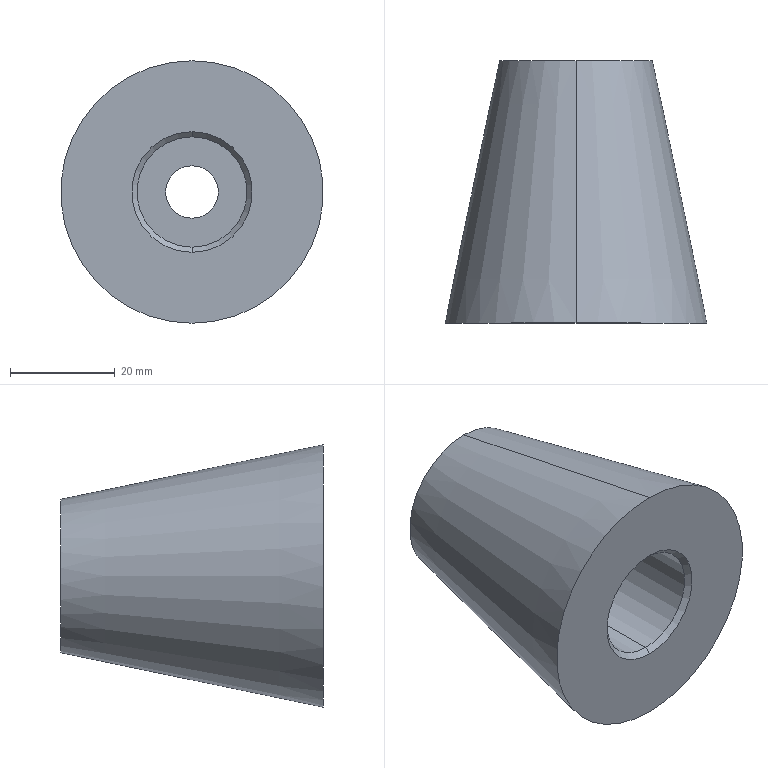Part | STEP file | ND25021-01-JDKM-05-SL | 1 solid | 13 faces | box 50 x 50 x 50 mm | volume 54211 mm3 | cone 6 | cylinder 4 | plane 3 | commonest cylinder face diameters 10 x2 21 x2
STEP:
#1=CARTESIAN_POINT('',(0.,0.,0.));
#2=DIRECTION('',(0.,0.,1.));
#3=DIRECTION('',(1.,0.,0.));
#4=AXIS2_PLACEMENT_3D('',#1,#2,#3);
#5=CARTESIAN_POINT('',(0.,1.,-10.5));
#6=VERTEX_POINT('',#5);
#7=CARTESIAN_POINT('',(0.,0.,-11.5));
#8=VERTEX_POINT('',#7);
#9=CARTESIAN_POINT('',(0.,1.,-10.5));
#10=DIRECTION('',(0.,-0.7071,-0.7071));
#11=VECTOR('',#10,1.);
#12=LINE('',#9,#11);
#13=CARTESIAN_POINT('',(0.,1.,0.));
#14=DIRECTION('',(0.,-1.,0.));
#15=DIRECTION('',(0.,0.,-1.));
#16=AXIS2_PLACEMENT_3D('',#13,#14,#15);
#17=CONICAL_SURFACE('',#16,10.5,0.7854);
#18=CARTESIAN_POINT('',(6.283,0.));
#19=DIRECTION('',(0.,1.));
#20=VECTOR('',#19,1.);
#21=LINE('',#18,#20);
#22=(GEOMETRIC_REPRESENTATION_CONTEXT(2)PARAMETRIC_REPRESENTATION_CONTEXT()REPRESENTATION_CONTEXT('',''));
#23=DEFINITIONAL_REPRESENTATION('',(#21),#22);
#24=PCURVE('',#17,#23);
#25=CARTESIAN_POINT('',(0.,1.,0.));
#26=DIRECTION('',(0.,-1.,0.));
#27=DIRECTION('',(0.,0.,-1.));
#28=AXIS2_PLACEMENT_3D('',#25,#26,#27);
#29=CONICAL_SURFACE('',#28,10.5,0.7854);
#30=CARTESIAN_POINT('',(0.,0.));
#31=DIRECTION('',(0.,1.));
#32=VECTOR('',#31,1.);
#33=LINE('',#30,#32);
#34=(GEOMETRIC_REPRESENTATION_CONTEXT(2)PARAMETRIC_REPRESENTATION_CONTEXT()REPRESENTATION_CONTEXT('',''));
#35=DEFINITIONAL_REPRESENTATION('',(#33),#34);
#36=PCURVE('',#29,#35);
#37=SURFACE_CURVE('',#12,(#24,#36),.PCURVE_S1.);
#38=EDGE_CURVE('',#6,#8,#37,.T.);
#39=ORIENTED_EDGE('',*,*,#38,.T.);
#40=CARTESIAN_POINT('',(0.,0.,11.5));
#41=VERTEX_POINT('',#40);
#42=CARTESIAN_POINT('',(0.,0.,0.));
#43=DIRECTION('',(0.,1.,0.));
#44=DIRECTION('',(0.,0.,1.));
#45=AXIS2_PLACEMENT_3D('',#42,#43,#44);
#46=CIRCLE('',#45,11.5);
#47=CARTESIAN_POINT('',(9.425,1.));
#48=DIRECTION('',(-1.,0.));
#49=VECTOR('',#48,1.);
#50=LINE('',#47,#49);
#51=(GEOMETRIC_REPRESENTATION_CONTEXT(2)PARAMETRIC_REPRESENTATION_CONTEXT()REPRESENTATION_CONTEXT('',''));
#52=DEFINITIONAL_REPRESENTATION('',(#50),#51);
#53=PCURVE('',#17,#52);
#54=CARTESIAN_POINT('',(0.,0.,0.));
#55=DIRECTION('',(0.,1.,0.));
#56=DIRECTION('',(0.,0.,1.));
#57=AXIS2_PLACEMENT_3D('',#54,#55,#56);
#58=PLANE('',#57);
#59=CARTESIAN_POINT('',(0.,0.));
#60=DIRECTION('',(1.,0.));
#61=AXIS2_PLACEMENT_2D('',#59,#60);
#62=CIRCLE('',#61,11.5);
#63=(GEOMETRIC_REPRESENTATION_CONTEXT(2)PARAMETRIC_REPRESENTATION_CONTEXT()REPRESENTATION_CONTEXT('',''));
#64=DEFINITIONAL_REPRESENTATION('',(#62),#63);
#65=PCURVE('',#58,#64);
#66=SURFACE_CURVE('',#46,(#53,#65),.PCURVE_S1.);
#67=EDGE_CURVE('',#8,#41,#66,.T.);
#68=ORIENTED_EDGE('',*,*,#67,.T.);
#69=CARTESIAN_POINT('',(0.,1.,10.5));
#70=VERTEX_POINT('',#69);
#71=CARTESIAN_POINT('',(0.,1.,10.5));
#72=DIRECTION('',(0.,-0.7071,0.7071));
#73=VECTOR('',#72,1.);
#74=LINE('',#71,#73);
#75=CARTESIAN_POINT('',(3.142,0.));
#76=DIRECTION('',(0.,1.));
#77=VECTOR('',#76,1.);
#78=LINE('',#75,#77);
#79=(GEOMETRIC_REPRESENTATION_CONTEXT(2)PARAMETRIC_REPRESENTATION_CONTEXT()REPRESENTATION_CONTEXT('',''));
#80=DEFINITIONAL_REPRESENTATION('',(#78),#79);
#81=PCURVE('',#17,#80);
#82=CARTESIAN_POINT('',(3.142,0.));
#83=DIRECTION('',(0.,1.));
#84=VECTOR('',#83,1.);
#85=LINE('',#82,#84);
#86=(GEOMETRIC_REPRESENTATION_CONTEXT(2)PARAMETRIC_REPRESENTATION_CONTEXT()REPRESENTATION_CONTEXT('',''));
#87=DEFINITIONAL_REPRESENTATION('',(#85),#86);
#88=PCURVE('',#29,#87);
#89=SURFACE_CURVE('',#74,(#81,#88),.PCURVE_S1.);
#90=EDGE_CURVE('',#70,#41,#89,.T.);
#91=ORIENTED_EDGE('',*,*,#90,.F.);
#92=CARTESIAN_POINT('',(0.,1.,0.));
#93=DIRECTION('',(0.,-1.,0.));
#94=DIRECTION('',(0.,0.,1.));
#95=AXIS2_PLACEMENT_3D('',#92,#93,#94);
#96=CIRCLE('',#95,10.5);
#97=CARTESIAN_POINT('',(3.142,0.));
#98=DIRECTION('',(1.,0.));
#99=VECTOR('',#98,1.);
#100=LINE('',#97,#99);
#101=(GEOMETRIC_REPRESENTATION_CONTEXT(2)PARAMETRIC_REPRESENTATION_CONTEXT()REPRESENTATION_CONTEXT('',''));
#102=DEFINITIONAL_REPRESENTATION('',(#100),#101);
#103=PCURVE('',#17,#102);
#104=CARTESIAN_POINT('',(0.,18.,0.));
#105=DIRECTION('',(0.,-1.,0.));
#106=DIRECTION('',(0.,0.,-1.));
#107=AXIS2_PLACEMENT_3D('',#104,#105,#106);
#108=CYLINDRICAL_SURFACE('',#107,10.5);
#109=CARTESIAN_POINT('',(3.142,17.));
#110=DIRECTION('',(1.,0.));
#111=VECTOR('',#110,1.);
#112=LINE('',#109,#111);
#113=(GEOMETRIC_REPRESENTATION_CONTEXT(2)PARAMETRIC_REPRESENTATION_CONTEXT()REPRESENTATION_CONTEXT('',''));
#114=DEFINITIONAL_REPRESENTATION('',(#112),#113);
#115=PCURVE('',#108,#114);
#116=SURFACE_CURVE('',#96,(#103,#115),.PCURVE_S1.);
#117=EDGE_CURVE('',#70,#6,#116,.T.);
#118=ORIENTED_EDGE('',*,*,#117,.T.);
#119=EDGE_LOOP('',(#39,#68,#91,#118));
#120=FACE_BOUND('',#119,.F.);
#121=ADVANCED_FACE('',(#120),#17,.F.);
#122=CARTESIAN_POINT('',(0.,18.,-10.5));
#123=VERTEX_POINT('',#122);
#124=CARTESIAN_POINT('',(0.,18.,-10.5));
#125=DIRECTION('',(0.,-1.,0.));
#126=VECTOR('',#125,1.);
#127=LINE('',#124,#126);
#128=CARTESIAN_POINT('',(6.283,0.));
#129=DIRECTION('',(0.,1.));
#130=VECTOR('',#129,1.);
#131=LINE('',#128,#130);
#132=(GEOMETRIC_REPRESENTATION_CONTEXT(2)PARAMETRIC_REPRESENTATION_CONTEXT()REPRESENTATION_CONTEXT('',''));
#133=DEFINITIONAL_REPRESENTATION('',(#131),#132);
#134=PCURVE('',#108,#133);
#135=CARTESIAN_POINT('',(0.,18.,0.));
#136=DIRECTION('',(0.,-1.,0.));
#137=DIRECTION('',(0.,0.,-1.));
#138=AXIS2_PLACEMENT_3D('',#135,#136,#137);
#139=CYLINDRICAL_SURFACE('',#138,10.5);
#140=CARTESIAN_POINT('',(0.,0.));
#141=DIRECTION('',(0.,1.));
#142=VECTOR('',#141,1.);
#143=LINE('',#140,#142);
#144=(GEOMETRIC_REPRESENTATION_CONTEXT(2)PARAMETRIC_REPRESENTATION_CONTEXT()REPRESENTATION_CONTEXT('',''));
#145=DEFINITIONAL_REPRESENTATION('',(#143),#144);
#146=PCURVE('',#139,#145);
#147=SURFACE_CURVE('',#127,(#134,#146),.PCURVE_S1.);
#148=EDGE_CURVE('',#123,#6,#147,.T.);
#149=ORIENTED_EDGE('',*,*,#148,.T.);
#150=ORIENTED_EDGE('',*,*,#117,.F.);
#151=CARTESIAN_POINT('',(0.,18.,10.5));
#152=VERTEX_POINT('',#151);
#153=CARTESIAN_POINT('',(0.,18.,10.5));
#154=DIRECTION('',(0.,-1.,0.));
#155=VECTOR('',#154,1.);
#156=LINE('',#153,#155);
#157=CARTESIAN_POINT('',(3.142,0.));
#158=DIRECTION('',(0.,1.));
#159=VECTOR('',#158,1.);
#160=LINE('',#157,#159);
#161=(GEOMETRIC_REPRESENTATION_CONTEXT(2)PARAMETRIC_REPRESENTATION_CONTEXT()REPRESENTATION_CONTEXT('',''));
#162=DEFINITIONAL_REPRESENTATION('',(#160),#161);
#163=PCURVE('',#108,#162);
#164=CARTESIAN_POINT('',(3.142,0.));
#165=DIRECTION('',(0.,1.));
#166=VECTOR('',#165,1.);
#167=LINE('',#164,#166);
#168=(GEOMETRIC_REPRESENTATION_CONTEXT(2)PARAMETRIC_REPRESENTATION_CONTEXT()REPRESENTATION_CONTEXT('',''));
#169=DEFINITIONAL_REPRESENTATION('',(#167),#168);
#170=PCURVE('',#139,#169);
#171=SURFACE_CURVE('',#156,(#163,#170),.PCURVE_S1.);
#172=EDGE_CURVE('',#152,#70,#171,.T.);
#173=ORIENTED_EDGE('',*,*,#172,.F.);
#174=CARTESIAN_POINT('',(0.,18.,0.));
#175=DIRECTION('',(0.,-1.,0.));
#176=DIRECTION('',(0.,0.,-1.));
#177=AXIS2_PLACEMENT_3D('',#174,#175,#176);
#178=CIRCLE('',#177,10.5);
#179=CARTESIAN_POINT('',(0.,0.));
#180=DIRECTION('',(1.,0.));
#181=VECTOR('',#180,1.);
#182=LINE('',#179,#181);
#183=(GEOMETRIC_REPRESENTATION_CONTEXT(2)PARAMETRIC_REPRESENTATION_CONTEXT()REPRESENTATION_CONTEXT('',''));
#184=DEFINITIONAL_REPRESENTATION('',(#182),#183);
#185=PCURVE('',#108,#184);
#186=CARTESIAN_POINT('',(0.,18.,0.));
#187=DIRECTION('',(0.,-1.,0.));
#188=DIRECTION('',(0.,0.,-1.));
#189=AXIS2_PLACEMENT_3D('',#186,#187,#188);
#190=PLANE('',#189);
#191=CARTESIAN_POINT('',(0.,0.));
#192=DIRECTION('',(1.,0.));
#193=AXIS2_PLACEMENT_2D('',#191,#192);
#194=CIRCLE('',#193,10.5);
#195=(GEOMETRIC_REPRESENTATION_CONTEXT(2)PARAMETRIC_REPRESENTATION_CONTEXT()REPRESENTATION_CONTEXT('',''));
#196=DEFINITIONAL_REPRESENTATION('',(#194),#195);
#197=PCURVE('',#190,#196);
#198=SURFACE_CURVE('',#178,(#185,#197),.PCURVE_S1.);
#199=EDGE_CURVE('',#152,#123,#198,.T.);
#200=ORIENTED_EDGE('',*,*,#199,.T.);
#201=EDGE_LOOP('',(#149,#150,#173,#200));
#202=FACE_BOUND('',#201,.F.);
#203=ADVANCED_FACE('',(#202),#108,.F.);
#204=CARTESIAN_POINT('',(0.,49.5,5.));
#205=VERTEX_POINT('',#204);
#206=CARTESIAN_POINT('',(0.,50.,5.5));
#207=VERTEX_POINT('',#206);
#208=CARTESIAN_POINT('',(0.,50.,5.5));
#209=DIRECTION('',(0.,0.7071,0.7071));
#210=VECTOR('',#209,1.);
#211=LINE('',#208,#210);
#212=CARTESIAN_POINT('',(0.,50.,0.));
#213=DIRECTION('',(0.,1.,0.));
#214=DIRECTION('',(0.,0.,1.));
#215=AXIS2_PLACEMENT_3D('',#212,#213,#214);
#216=CONICAL_SURFACE('',#215,5.5,0.7854);
#217=CARTESIAN_POINT('',(6.283,0.));
#218=DIRECTION('',(0.,1.));
#219=VECTOR('',#218,1.);
#220=LINE('',#217,#219);
#221=(GEOMETRIC_REPRESENTATION_CONTEXT(2)PARAMETRIC_REPRESENTATION_CONTEXT()REPRESENTATION_CONTEXT('',''));
#222=DEFINITIONAL_REPRESENTATION('',(#220),#221);
#223=PCURVE('',#216,#222);
#224=CARTESIAN_POINT('',(0.,50.,0.));
#225=DIRECTION('',(0.,1.,0.));
#226=DIRECTION('',(0.,0.,1.));
#227=AXIS2_PLACEMENT_3D('',#224,#225,#226);
#228=CONICAL_SURFACE('',#227,5.5,0.7854);
#229=CARTESIAN_POINT('',(0.,0.));
#230=DIRECTION('',(0.,1.));
#231=VECTOR('',#230,1.);
#232=LINE('',#229,#231);
#233=(GEOMETRIC_REPRESENTATION_CONTEXT(2)PARAMETRIC_REPRESENTATION_CONTEXT()REPRESENTATION_CONTEXT('',''));
#234=DEFINITIONAL_REPRESENTATION('',(#232),#233);
#235=PCURVE('',#228,#234);
#236=SURFACE_CURVE('',#211,(#223,#235),.PCURVE_S1.);
#237=EDGE_CURVE('',#205,#207,#236,.T.);
#238=ORIENTED_EDGE('',*,*,#237,.T.);
#239=CARTESIAN_POINT('',(0.,50.,-5.5));
#240=VERTEX_POINT('',#239);
#241=CARTESIAN_POINT('',(0.,50.,0.));
#242=DIRECTION('',(0.,-1.,0.));
#243=DIRECTION('',(0.,0.,1.));
#244=AXIS2_PLACEMENT_3D('',#241,#242,#243);
#245=CIRCLE('',#244,5.5);
#246=CARTESIAN_POINT('',(6.283,0.));
#247=DIRECTION('',(-1.,0.));
#248=VECTOR('',#247,1.);
#249=LINE('',#246,#248);
#250=(GEOMETRIC_REPRESENTATION_CONTEXT(2)PARAMETRIC_REPRESENTATION_CONTEXT()REPRESENTATION_CONTEXT('',''));
#251=DEFINITIONAL_REPRESENTATION('',(#249),#250);
#252=PCURVE('',#216,#251);
#253=CARTESIAN_POINT('',(0.,50.,0.));
#254=DIRECTION('',(0.,1.,0.));
#255=DIRECTION('',(0.,0.,1.));
#256=AXIS2_PLACEMENT_3D('',#253,#254,#255);
#257=PLANE('',#256);
#258=CARTESIAN_POINT('',(5.5,0.));
#259=CARTESIAN_POINT('',(5.5,-9.526));
#260=CARTESIAN_POINT('',(-2.75,-4.763));
#261=CARTESIAN_POINT('',(-11.,0.));
#262=CARTESIAN_POINT('',(-2.75,4.763));
#263=CARTESIAN_POINT('',(5.5,9.526));
#264=CARTESIAN_POINT('',(5.5,0.));
#265=(BOUNDED_CURVE()B_SPLINE_CURVE(2,(#258,#259,#260,#261,#262,#263,#264),.UNSPECIFIED.,.T.,.F.)B_SPLINE_CURVE_WITH_KNOTS((1,2,2,2,2,1),(-2.094,0.,2.094,4.189,6.283,8.378),.UNSPECIFIED.)CURVE()GEOMETRIC_REPRESENTATION_ITEM()RATIONAL_B_SPLINE_CURVE((1.,0.5,1.,0.5,1.,0.5,1.))REPRESENTATION_ITEM(''));
#266=(GEOMETRIC_REPRESENTATION_CONTEXT(2)PARAMETRIC_REPRESENTATION_CONTEXT()REPRESENTATION_CONTEXT('',''));
#267=DEFINITIONAL_REPRESENTATION('',(#265),#266);
#268=PCURVE('',#257,#267);
#269=SURFACE_CURVE('',#245,(#252,#268),.PCURVE_S1.);
#270=EDGE_CURVE('',#207,#240,#269,.T.);
#271=ORIENTED_EDGE('',*,*,#270,.T.);
#272=CARTESIAN_POINT('',(0.,49.5,-5.));
#273=VERTEX_POINT('',#272);
#274=CARTESIAN_POINT('',(0.,50.,-5.5));
#275=DIRECTION('',(0.,0.7071,-0.7071));
#276=VECTOR('',#275,1.);
#277=LINE('',#274,#276);
#278=CARTESIAN_POINT('',(3.142,0.));
#279=DIRECTION('',(0.,1.));
#280=VECTOR('',#279,1.);
#281=LINE('',#278,#280);
#282=(GEOMETRIC_REPRESENTATION_CONTEXT(2)PARAMETRIC_REPRESENTATION_CONTEXT()REPRESENTATION_CONTEXT('',''));
#283=DEFINITIONAL_REPRESENTATION('',(#281),#282);
#284=PCURVE('',#216,#283);
#285=CARTESIAN_POINT('',(3.142,0.));
#286=DIRECTION('',(0.,1.));
#287=VECTOR('',#286,1.);
#288=LINE('',#285,#287);
#289=(GEOMETRIC_REPRESENTATION_CONTEXT(2)PARAMETRIC_REPRESENTATION_CONTEXT()REPRESENTATION_CONTEXT('',''));
#290=DEFINITIONAL_REPRESENTATION('',(#288),#289);
#291=PCURVE('',#228,#290);
#292=SURFACE_CURVE('',#277,(#284,#291),.PCURVE_S1.);
#293=EDGE_CURVE('',#273,#240,#292,.T.);
#294=ORIENTED_EDGE('',*,*,#293,.F.);
#295=CARTESIAN_POINT('',(0.,49.5,0.));
#296=DIRECTION('',(0.,1.,0.));
#297=DIRECTION('',(0.,0.,1.));
#298=AXIS2_PLACEMENT_3D('',#295,#296,#297);
#299=CIRCLE('',#298,5.);
#300=CARTESIAN_POINT('',(0.,-0.5));
#301=DIRECTION('',(1.,0.));
#302=VECTOR('',#301,1.);
#303=LINE('',#300,#302);
#304=(GEOMETRIC_REPRESENTATION_CONTEXT(2)PARAMETRIC_REPRESENTATION_CONTEXT()REPRESENTATION_CONTEXT('',''));
#305=DEFINITIONAL_REPRESENTATION('',(#303),#304);
#306=PCURVE('',#216,#305);
#307=CARTESIAN_POINT('',(0.,50.,0.));
#308=DIRECTION('',(0.,-1.,0.));
#309=DIRECTION('',(0.,0.,-1.));
#310=AXIS2_PLACEMENT_3D('',#307,#308,#309);
#311=CYLINDRICAL_SURFACE('',#310,5.);
#312=CARTESIAN_POINT('',(9.425,0.5));
#313=DIRECTION('',(-1.,0.));
#314=VECTOR('',#313,1.);
#315=LINE('',#312,#314);
#316=(GEOMETRIC_REPRESENTATION_CONTEXT(2)PARAMETRIC_REPRESENTATION_CONTEXT()REPRESENTATION_CONTEXT('',''));
#317=DEFINITIONAL_REPRESENTATION('',(#315),#316);
#318=PCURVE('',#311,#317);
#319=SURFACE_CURVE('',#299,(#306,#318),.PCURVE_S1.);
#320=EDGE_CURVE('',#273,#205,#319,.T.);
#321=ORIENTED_EDGE('',*,*,#320,.T.);
#322=EDGE_LOOP('',(#238,#271,#294,#321));
#323=FACE_BOUND('',#322,.F.);
#324=ADVANCED_FACE('',(#323),#216,.F.);
#325=CARTESIAN_POINT('',(0.,50.,14.6));
#326=VERTEX_POINT('',#325);
#327=CARTESIAN_POINT('',(0.,50.,-14.6));
#328=VERTEX_POINT('',#327);
#329=CARTESIAN_POINT('',(0.,50.,0.));
#330=DIRECTION('',(0.,1.,0.));
#331=DIRECTION('',(0.,0.,1.));
#332=AXIS2_PLACEMENT_3D('',#329,#330,#331);
#333=CIRCLE('',#332,14.6);
#334=CARTESIAN_POINT('',(0.,50.,0.));
#335=DIRECTION('',(0.,-1.,0.));
#336=DIRECTION('',(0.,0.,-1.));
#337=AXIS2_PLACEMENT_3D('',#334,#335,#336);
#338=CONICAL_SURFACE('',#337,14.6,0.2051);
#339=CARTESIAN_POINT('',(3.142,0.));
#340=DIRECTION('',(-1.,0.));
#341=VECTOR('',#340,1.);
#342=LINE('',#339,#341);
#343=(GEOMETRIC_REPRESENTATION_CONTEXT(2)PARAMETRIC_REPRESENTATION_CONTEXT()REPRESENTATION_CONTEXT('',''));
#344=DEFINITIONAL_REPRESENTATION('',(#342),#343);
#345=PCURVE('',#338,#344);
#346=CARTESIAN_POINT('',(0.,0.));
#347=DIRECTION('',(1.,0.));
#348=AXIS2_PLACEMENT_2D('',#346,#347);
#349=CIRCLE('',#348,14.6);
#350=(GEOMETRIC_REPRESENTATION_CONTEXT(2)PARAMETRIC_REPRESENTATION_CONTEXT()REPRESENTATION_CONTEXT('',''));
#351=DEFINITIONAL_REPRESENTATION('',(#349),#350);
#352=PCURVE('',#257,#351);
#353=SURFACE_CURVE('',#333,(#345,#352),.PCURVE_S1.);
#354=EDGE_CURVE('',#326,#328,#353,.T.);
#355=ORIENTED_EDGE('',*,*,#354,.F.);
#356=CARTESIAN_POINT('',(0.,0.,25.));
#357=VERTEX_POINT('',#356);
#358=CARTESIAN_POINT('',(0.,50.,14.6));
#359=DIRECTION('',(0.,-0.979,0.2036));
#360=VECTOR('',#359,1.);
#361=LINE('',#358,#360);
#362=CARTESIAN_POINT('',(3.142,0.));
#363=DIRECTION('',(0.,1.));
#364=VECTOR('',#363,1.);
#365=LINE('',#362,#364);
#366=(GEOMETRIC_REPRESENTATION_CONTEXT(2)PARAMETRIC_REPRESENTATION_CONTEXT()REPRESENTATION_CONTEXT('',''));
#367=DEFINITIONAL_REPRESENTATION('',(#365),#366);
#368=PCURVE('',#338,#367);
#369=CARTESIAN_POINT('',(0.,50.,0.));
#370=DIRECTION('',(0.,-1.,0.));
#371=DIRECTION('',(0.,0.,-1.));
#372=AXIS2_PLACEMENT_3D('',#369,#370,#371);
#373=CONICAL_SURFACE('',#372,14.6,0.2051);
#374=CARTESIAN_POINT('',(3.142,0.));
#375=DIRECTION('',(0.,1.));
#376=VECTOR('',#375,1.);
#377=LINE('',#374,#376);
#378=(GEOMETRIC_REPRESENTATION_CONTEXT(2)PARAMETRIC_REPRESENTATION_CONTEXT()REPRESENTATION_CONTEXT('',''));
#379=DEFINITIONAL_REPRESENTATION('',(#377),#378);
#380=PCURVE('',#373,#379);
#381=SURFACE_CURVE('',#361,(#368,#380),.PCURVE_S1.);
#382=EDGE_CURVE('',#326,#357,#381,.T.);
#383=ORIENTED_EDGE('',*,*,#382,.T.);
#384=CARTESIAN_POINT('',(0.,0.,-25.));
#385=VERTEX_POINT('',#384);
#386=CARTESIAN_POINT('',(0.,0.,0.));
#387=DIRECTION('',(0.,1.,0.));
#388=DIRECTION('',(0.,0.,1.));
#389=AXIS2_PLACEMENT_3D('',#386,#387,#388);
#390=CIRCLE('',#389,25.);
#391=CARTESIAN_POINT('',(3.142,50.));
#392=DIRECTION('',(-1.,0.));
#393=VECTOR('',#392,1.);
#394=LINE('',#391,#393);
#395=(GEOMETRIC_REPRESENTATION_CONTEXT(2)PARAMETRIC_REPRESENTATION_CONTEXT()REPRESENTATION_CONTEXT('',''));
#396=DEFINITIONAL_REPRESENTATION('',(#394),#395);
#397=PCURVE('',#338,#396);
#398=CARTESIAN_POINT('',(0.,0.));
#399=DIRECTION('',(1.,0.));
#400=AXIS2_PLACEMENT_2D('',#398,#399);
#401=CIRCLE('',#400,25.);
#402=(GEOMETRIC_REPRESENTATION_CONTEXT(2)PARAMETRIC_REPRESENTATION_CONTEXT()REPRESENTATION_CONTEXT('',''));
#403=DEFINITIONAL_REPRESENTATION('',(#401),#402);
#404=PCURVE('',#58,#403);
#405=SURFACE_CURVE('',#390,(#397,#404),.PCURVE_S1.);
#406=EDGE_CURVE('',#357,#385,#405,.T.);
#407=ORIENTED_EDGE('',*,*,#406,.T.);
#408=CARTESIAN_POINT('',(0.,50.,-14.6));
#409=DIRECTION('',(0.,-0.979,-0.2036));
#410=VECTOR('',#409,1.);
#411=LINE('',#408,#410);
#412=CARTESIAN_POINT('',(0.,0.));
#413=DIRECTION('',(0.,1.));
#414=VECTOR('',#413,1.);
#415=LINE('',#412,#414);
#416=(GEOMETRIC_REPRESENTATION_CONTEXT(2)PARAMETRIC_REPRESENTATION_CONTEXT()REPRESENTATION_CONTEXT('',''));
#417=DEFINITIONAL_REPRESENTATION('',(#415),#416);
#418=PCURVE('',#338,#417);
#419=CARTESIAN_POINT('',(6.283,0.));
#420=DIRECTION('',(0.,1.));
#421=VECTOR('',#420,1.);
#422=LINE('',#419,#421);
#423=(GEOMETRIC_REPRESENTATION_CONTEXT(2)PARAMETRIC_REPRESENTATION_CONTEXT()REPRESENTATION_CONTEXT('',''));
#424=DEFINITIONAL_REPRESENTATION('',(#422),#423);
#425=PCURVE('',#373,#424);
#426=SURFACE_CURVE('',#411,(#418,#425),.PCURVE_S1.);
#427=EDGE_CURVE('',#328,#385,#426,.T.);
#428=ORIENTED_EDGE('',*,*,#427,.F.);
#429=EDGE_LOOP('',(#355,#383,#407,#428));
#430=FACE_BOUND('',#429,.T.);
#431=ADVANCED_FACE('',(#430),#338,.T.);
#432=CARTESIAN_POINT('',(0.,18.,-5.));
#433=VERTEX_POINT('',#432);
#434=CARTESIAN_POINT('',(0.,50.,-5.));
#435=DIRECTION('',(0.,-1.,0.));
#436=VECTOR('',#435,1.);
#437=LINE('',#434,#436);
#438=CARTESIAN_POINT('',(6.283,0.));
#439=DIRECTION('',(0.,1.));
#440=VECTOR('',#439,1.);
#441=LINE('',#438,#440);
#442=(GEOMETRIC_REPRESENTATION_CONTEXT(2)PARAMETRIC_REPRESENTATION_CONTEXT()REPRESENTATION_CONTEXT('',''));
#443=DEFINITIONAL_REPRESENTATION('',(#441),#442);
#444=PCURVE('',#311,#443);
#445=CARTESIAN_POINT('',(0.,50.,0.));
#446=DIRECTION('',(0.,-1.,0.));
#447=DIRECTION('',(0.,0.,-1.));
#448=AXIS2_PLACEMENT_3D('',#445,#446,#447);
#449=CYLINDRICAL_SURFACE('',#448,5.);
#450=CARTESIAN_POINT('',(0.,0.));
#451=DIRECTION('',(0.,1.));
#452=VECTOR('',#451,1.);
#453=LINE('',#450,#452);
#454=(GEOMETRIC_REPRESENTATION_CONTEXT(2)PARAMETRIC_REPRESENTATION_CONTEXT()REPRESENTATION_CONTEXT('',''));
#455=DEFINITIONAL_REPRESENTATION('',(#453),#454);
#456=PCURVE('',#449,#455);
#457=SURFACE_CURVE('',#437,(#444,#456),.PCURVE_S1.);
#458=EDGE_CURVE('',#273,#433,#457,.T.);
#459=ORIENTED_EDGE('',*,*,#458,.T.);
#460=CARTESIAN_POINT('',(0.,18.,5.));
#461=VERTEX_POINT('',#460);
#462=CARTESIAN_POINT('',(0.,18.,0.));
#463=DIRECTION('',(0.,1.,0.));
#464=DIRECTION('',(0.,0.,-1.));
#465=AXIS2_PLACEMENT_3D('',#462,#463,#464);
#466=CIRCLE('',#465,5.);
#467=CARTESIAN_POINT('',(6.283,32.));
#468=DIRECTION('',(-1.,0.));
#469=VECTOR('',#468,1.);
#470=LINE('',#467,#469);
#471=(GEOMETRIC_REPRESENTATION_CONTEXT(2)PARAMETRIC_REPRESENTATION_CONTEXT()REPRESENTATION_CONTEXT('',''));
#472=DEFINITIONAL_REPRESENTATION('',(#470),#471);
#473=PCURVE('',#311,#472);
#474=CARTESIAN_POINT('',(5.,0.));
#475=CARTESIAN_POINT('',(5.,-8.66));
#476=CARTESIAN_POINT('',(-2.5,-4.33));
#477=CARTESIAN_POINT('',(-10.,0.));
#478=CARTESIAN_POINT('',(-2.5,4.33));
#479=CARTESIAN_POINT('',(5.,8.66));
#480=CARTESIAN_POINT('',(5.,0.));
#481=(BOUNDED_CURVE()B_SPLINE_CURVE(2,(#474,#475,#476,#477,#478,#479,#480),.UNSPECIFIED.,.T.,.F.)B_SPLINE_CURVE_WITH_KNOTS((1,2,2,2,2,1),(-2.094,0.,2.094,4.189,6.283,8.378),.UNSPECIFIED.)CURVE()GEOMETRIC_REPRESENTATION_ITEM()RATIONAL_B_SPLINE_CURVE((1.,0.5,1.,0.5,1.,0.5,1.))REPRESENTATION_ITEM(''));
#482=(GEOMETRIC_REPRESENTATION_CONTEXT(2)PARAMETRIC_REPRESENTATION_CONTEXT()REPRESENTATION_CONTEXT('',''));
#483=DEFINITIONAL_REPRESENTATION('',(#481),#482);
#484=PCURVE('',#190,#483);
#485=SURFACE_CURVE('',#466,(#473,#484),.PCURVE_S1.);
#486=EDGE_CURVE('',#433,#461,#485,.T.);
#487=ORIENTED_EDGE('',*,*,#486,.T.);
#488=CARTESIAN_POINT('',(0.,50.,5.));
#489=DIRECTION('',(0.,-1.,0.));
#490=VECTOR('',#489,1.);
#491=LINE('',#488,#490);
#492=CARTESIAN_POINT('',(3.142,0.));
#493=DIRECTION('',(0.,1.));
#494=VECTOR('',#493,1.);
#495=LINE('',#492,#494);
#496=(GEOMETRIC_REPRESENTATION_CONTEXT(2)PARAMETRIC_REPRESENTATION_CONTEXT()REPRESENTATION_CONTEXT('',''));
#497=DEFINITIONAL_REPRESENTATION('',(#495),#496);
#498=PCURVE('',#311,#497);
#499=CARTESIAN_POINT('',(3.142,0.));
#500=DIRECTION('',(0.,1.));
#501=VECTOR('',#500,1.);
#502=LINE('',#499,#501);
#503=(GEOMETRIC_REPRESENTATION_CONTEXT(2)PARAMETRIC_REPRESENTATION_CONTEXT()REPRESENTATION_CONTEXT('',''));
#504=DEFINITIONAL_REPRESENTATION('',(#502),#503);
#505=PCURVE('',#449,#504);
#506=SURFACE_CURVE('',#491,(#498,#505),.PCURVE_S1.);
#507=EDGE_CURVE('',#205,#461,#506,.T.);
#508=ORIENTED_EDGE('',*,*,#507,.F.);
#509=ORIENTED_EDGE('',*,*,#320,.F.);
#510=EDGE_LOOP('',(#459,#487,#508,#509));
#511=FACE_BOUND('',#510,.F.);
#512=ADVANCED_FACE('',(#511),#311,.F.);
#513=CARTESIAN_POINT('',(0.,18.,0.));
#514=DIRECTION('',(0.,1.,0.));
#515=DIRECTION('',(0.,0.,-1.));
#516=AXIS2_PLACEMENT_3D('',#513,#514,#515);
#517=CIRCLE('',#516,5.);
#518=CARTESIAN_POINT('',(6.283,32.));
#519=DIRECTION('',(-1.,0.));
#520=VECTOR('',#519,1.);
#521=LINE('',#518,#520);
#522=(GEOMETRIC_REPRESENTATION_CONTEXT(2)PARAMETRIC_REPRESENTATION_CONTEXT()REPRESENTATION_CONTEXT('',''));
#523=DEFINITIONAL_REPRESENTATION('',(#521),#522);
#524=PCURVE('',#449,#523);
#525=CARTESIAN_POINT('',(5.,0.));
#526=CARTESIAN_POINT('',(5.,-8.66));
#527=CARTESIAN_POINT('',(-2.5,-4.33));
#528=CARTESIAN_POINT('',(-10.,0.));
#529=CARTESIAN_POINT('',(-2.5,4.33));
#530=CARTESIAN_POINT('',(5.,8.66));
#531=CARTESIAN_POINT('',(5.,0.));
#532=(BOUNDED_CURVE()B_SPLINE_CURVE(2,(#525,#526,#527,#528,#529,#530,#531),.UNSPECIFIED.,.T.,.F.)B_SPLINE_CURVE_WITH_KNOTS((1,2,2,2,2,1),(-2.094,0.,2.094,4.189,6.283,8.378),.UNSPECIFIED.)CURVE()GEOMETRIC_REPRESENTATION_ITEM()RATIONAL_B_SPLINE_CURVE((1.,0.5,1.,0.5,1.,0.5,1.))REPRESENTATION_ITEM(''));
#533=(GEOMETRIC_REPRESENTATION_CONTEXT(2)PARAMETRIC_REPRESENTATION_CONTEXT()REPRESENTATION_CONTEXT('',''));
#534=DEFINITIONAL_REPRESENTATION('',(#532),#533);
#535=PCURVE('',#190,#534);
#536=SURFACE_CURVE('',#517,(#524,#535),.PCURVE_S1.);
#537=EDGE_CURVE('',#461,#433,#536,.T.);
#538=ORIENTED_EDGE('',*,*,#537,.T.);
#539=ORIENTED_EDGE('',*,*,#458,.F.);
#540=CARTESIAN_POINT('',(0.,49.5,0.));
#541=DIRECTION('',(0.,1.,0.));
#542=DIRECTION('',(0.,0.,1.));
#543=AXIS2_PLACEMENT_3D('',#540,#541,#542);
#544=CIRCLE('',#543,5.);
#545=CARTESIAN_POINT('',(3.142,0.5));
#546=DIRECTION('',(-1.,0.));
#547=VECTOR('',#546,1.);
#548=LINE('',#545,#547);
#549=(GEOMETRIC_REPRESENTATION_CONTEXT(2)PARAMETRIC_REPRESENTATION_CONTEXT()REPRESENTATION_CONTEXT('',''));
#550=DEFINITIONAL_REPRESENTATION('',(#548),#549);
#551=PCURVE('',#449,#550);
#552=CARTESIAN_POINT('',(0.,-0.5));
#553=DIRECTION('',(1.,0.));
#554=VECTOR('',#553,1.);
#555=LINE('',#552,#554);
#556=(GEOMETRIC_REPRESENTATION_CONTEXT(2)PARAMETRIC_REPRESENTATION_CONTEXT()REPRESENTATION_CONTEXT('',''));
#557=DEFINITIONAL_REPRESENTATION('',(#555),#556);
#558=PCURVE('',#228,#557);
#559=SURFACE_CURVE('',#544,(#551,#558),.PCURVE_S1.);
#560=EDGE_CURVE('',#205,#273,#559,.T.);
#561=ORIENTED_EDGE('',*,*,#560,.F.);
#562=ORIENTED_EDGE('',*,*,#507,.T.);
#563=EDGE_LOOP('',(#538,#539,#561,#562));
#564=FACE_BOUND('',#563,.F.);
#565=ADVANCED_FACE('',(#564),#449,.F.);
#566=ORIENTED_EDGE('',*,*,#270,.T.);
#567=CARTESIAN_POINT('',(0.,50.,0.));
#568=DIRECTION('',(0.,-1.,0.));
#569=DIRECTION('',(0.,0.,1.));
#570=AXIS2_PLACEMENT_3D('',#567,#568,#569);
#571=CIRCLE('',#570,5.5);
#572=CARTESIAN_POINT('',(5.5,0.));
#573=CARTESIAN_POINT('',(5.5,-9.526));
#574=CARTESIAN_POINT('',(-2.75,-4.763));
#575=CARTESIAN_POINT('',(-11.,0.));
#576=CARTESIAN_POINT('',(-2.75,4.763));
#577=CARTESIAN_POINT('',(5.5,9.526));
#578=CARTESIAN_POINT('',(5.5,0.));
#579=(BOUNDED_CURVE()B_SPLINE_CURVE(2,(#572,#573,#574,#575,#576,#577,#578),.UNSPECIFIED.,.T.,.F.)B_SPLINE_CURVE_WITH_KNOTS((1,2,2,2,2,1),(-2.094,0.,2.094,4.189,6.283,8.378),.UNSPECIFIED.)CURVE()GEOMETRIC_REPRESENTATION_ITEM()RATIONAL_B_SPLINE_CURVE((1.,0.5,1.,0.5,1.,0.5,1.))REPRESENTATION_ITEM(''));
#580=(GEOMETRIC_REPRESENTATION_CONTEXT(2)PARAMETRIC_REPRESENTATION_CONTEXT()REPRESENTATION_CONTEXT('',''));
#581=DEFINITIONAL_REPRESENTATION('',(#579),#580);
#582=PCURVE('',#257,#581);
#583=CARTESIAN_POINT('',(6.283,0.));
#584=DIRECTION('',(-1.,0.));
#585=VECTOR('',#584,1.);
#586=LINE('',#583,#585);
#587=(GEOMETRIC_REPRESENTATION_CONTEXT(2)PARAMETRIC_REPRESENTATION_CONTEXT()REPRESENTATION_CONTEXT('',''));
#588=DEFINITIONAL_REPRESENTATION('',(#586),#587);
#589=PCURVE('',#228,#588);
#590=SURFACE_CURVE('',#571,(#582,#589),.PCURVE_S1.);
#591=EDGE_CURVE('',#240,#207,#590,.T.);
#592=ORIENTED_EDGE('',*,*,#591,.T.);
#593=EDGE_LOOP('',(#566,#592));
#594=FACE_BOUND('',#593,.T.);
#595=CARTESIAN_POINT('',(0.,50.,0.));
#596=DIRECTION('',(0.,1.,0.));
#597=DIRECTION('',(0.,0.,1.));
#598=AXIS2_PLACEMENT_3D('',#595,#596,#597);
#599=CIRCLE('',#598,14.6);
#600=CARTESIAN_POINT('',(0.,0.));
#601=DIRECTION('',(1.,0.));
#602=AXIS2_PLACEMENT_2D('',#600,#601);
#603=CIRCLE('',#602,14.6);
#604=(GEOMETRIC_REPRESENTATION_CONTEXT(2)PARAMETRIC_REPRESENTATION_CONTEXT()REPRESENTATION_CONTEXT('',''));
#605=DEFINITIONAL_REPRESENTATION('',(#603),#604);
#606=PCURVE('',#257,#605);
#607=CARTESIAN_POINT('',(9.425,0.));
#608=DIRECTION('',(-1.,0.));
#609=VECTOR('',#608,1.);
#610=LINE('',#607,#609);
#611=(GEOMETRIC_REPRESENTATION_CONTEXT(2)PARAMETRIC_REPRESENTATION_CONTEXT()REPRESENTATION_CONTEXT('',''));
#612=DEFINITIONAL_REPRESENTATION('',(#610),#611);
#613=PCURVE('',#373,#612);
#614=SURFACE_CURVE('',#599,(#606,#613),.PCURVE_S1.);
#615=EDGE_CURVE('',#328,#326,#614,.T.);
#616=ORIENTED_EDGE('',*,*,#615,.T.);
#617=ORIENTED_EDGE('',*,*,#354,.T.);
#618=EDGE_LOOP('',(#616,#617));
#619=FACE_BOUND('',#618,.T.);
#620=ADVANCED_FACE('',(#594,#619),#257,.T.);
#621=ORIENTED_EDGE('',*,*,#67,.T.);
#622=CARTESIAN_POINT('',(0.,0.,0.));
#623=DIRECTION('',(0.,1.,0.));
#624=DIRECTION('',(0.,0.,1.));
#625=AXIS2_PLACEMENT_3D('',#622,#623,#624);
#626=CIRCLE('',#625,11.5);
#627=CARTESIAN_POINT('',(0.,0.));
#628=DIRECTION('',(1.,0.));
#629=AXIS2_PLACEMENT_2D('',#627,#628);
#630=CIRCLE('',#629,11.5);
#631=(GEOMETRIC_REPRESENTATION_CONTEXT(2)PARAMETRIC_REPRESENTATION_CONTEXT()REPRESENTATION_CONTEXT('',''));
#632=DEFINITIONAL_REPRESENTATION('',(#630),#631);
#633=PCURVE('',#58,#632);
#634=CARTESIAN_POINT('',(3.142,1.));
#635=DIRECTION('',(-1.,0.));
#636=VECTOR('',#635,1.);
#637=LINE('',#634,#636);
#638=(GEOMETRIC_REPRESENTATION_CONTEXT(2)PARAMETRIC_REPRESENTATION_CONTEXT()REPRESENTATION_CONTEXT('',''));
#639=DEFINITIONAL_REPRESENTATION('',(#637),#638);
#640=PCURVE('',#29,#639);
#641=SURFACE_CURVE('',#626,(#633,#640),.PCURVE_S1.);
#642=EDGE_CURVE('',#41,#8,#641,.T.);
#643=ORIENTED_EDGE('',*,*,#642,.T.);
#644=EDGE_LOOP('',(#621,#643));
#645=FACE_BOUND('',#644,.T.);
#646=CARTESIAN_POINT('',(0.,0.,0.));
#647=DIRECTION('',(0.,1.,0.));
#648=DIRECTION('',(0.,0.,1.));
#649=AXIS2_PLACEMENT_3D('',#646,#647,#648);
#650=CIRCLE('',#649,25.);
#651=CARTESIAN_POINT('',(0.,0.));
#652=DIRECTION('',(1.,0.));
#653=AXIS2_PLACEMENT_2D('',#651,#652);
#654=CIRCLE('',#653,25.);
#655=(GEOMETRIC_REPRESENTATION_CONTEXT(2)PARAMETRIC_REPRESENTATION_CONTEXT()REPRESENTATION_CONTEXT('',''));
#656=DEFINITIONAL_REPRESENTATION('',(#654),#655);
#657=PCURVE('',#58,#656);
#658=CARTESIAN_POINT('',(9.425,50.));
#659=DIRECTION('',(-1.,0.));
#660=VECTOR('',#659,1.);
#661=LINE('',#658,#660);
#662=(GEOMETRIC_REPRESENTATION_CONTEXT(2)PARAMETRIC_REPRESENTATION_CONTEXT()REPRESENTATION_CONTEXT('',''));
#663=DEFINITIONAL_REPRESENTATION('',(#661),#662);
#664=PCURVE('',#373,#663);
#665=SURFACE_CURVE('',#650,(#657,#664),.PCURVE_S1.);
#666=EDGE_CURVE('',#385,#357,#665,.T.);
#667=ORIENTED_EDGE('',*,*,#666,.F.);
#668=ORIENTED_EDGE('',*,*,#406,.F.);
#669=EDGE_LOOP('',(#667,#668));
#670=FACE_BOUND('',#669,.T.);
#671=ADVANCED_FACE('',(#645,#670),#58,.F.);
#672=ORIENTED_EDGE('',*,*,#382,.F.);
#673=ORIENTED_EDGE('',*,*,#615,.F.);
#674=ORIENTED_EDGE('',*,*,#427,.T.);
#675=ORIENTED_EDGE('',*,*,#666,.T.);
#676=EDGE_LOOP('',(#672,#673,#674,#675));
#677=FACE_BOUND('',#676,.T.);
#678=ADVANCED_FACE('',(#677),#373,.T.);
#679=ORIENTED_EDGE('',*,*,#591,.T.);
#680=ORIENTED_EDGE('',*,*,#237,.F.);
#681=ORIENTED_EDGE('',*,*,#560,.T.);
#682=ORIENTED_EDGE('',*,*,#293,.T.);
#683=EDGE_LOOP('',(#679,#680,#681,#682));
#684=FACE_BOUND('',#683,.F.);
#685=ADVANCED_FACE('',(#684),#228,.F.);
#686=CARTESIAN_POINT('',(0.,18.,0.));
#687=DIRECTION('',(0.,-1.,0.));
#688=DIRECTION('',(0.,0.,-1.));
#689=AXIS2_PLACEMENT_3D('',#686,#687,#688);
#690=CIRCLE('',#689,10.5);
#691=CARTESIAN_POINT('',(0.,0.));
#692=DIRECTION('',(1.,0.));
#693=AXIS2_PLACEMENT_2D('',#691,#692);
#694=CIRCLE('',#693,10.5);
#695=(GEOMETRIC_REPRESENTATION_CONTEXT(2)PARAMETRIC_REPRESENTATION_CONTEXT()REPRESENTATION_CONTEXT('',''));
#696=DEFINITIONAL_REPRESENTATION('',(#694),#695);
#697=PCURVE('',#190,#696);
#698=CARTESIAN_POINT('',(0.,0.));
#699=DIRECTION('',(1.,0.));
#700=VECTOR('',#699,1.);
#701=LINE('',#698,#700);
#702=(GEOMETRIC_REPRESENTATION_CONTEXT(2)PARAMETRIC_REPRESENTATION_CONTEXT()REPRESENTATION_CONTEXT('',''));
#703=DEFINITIONAL_REPRESENTATION('',(#701),#702);
#704=PCURVE('',#139,#703);
#705=SURFACE_CURVE('',#690,(#697,#704),.PCURVE_S1.);
#706=EDGE_CURVE('',#123,#152,#705,.T.);
#707=ORIENTED_EDGE('',*,*,#706,.T.);
#708=ORIENTED_EDGE('',*,*,#199,.T.);
#709=EDGE_LOOP('',(#707,#708));
#710=FACE_BOUND('',#709,.T.);
#711=ORIENTED_EDGE('',*,*,#486,.T.);
#712=ORIENTED_EDGE('',*,*,#537,.T.);
#713=EDGE_LOOP('',(#711,#712));
#714=FACE_BOUND('',#713,.T.);
#715=ADVANCED_FACE('',(#710,#714),#190,.T.);
#716=CARTESIAN_POINT('',(0.,1.,0.));
#717=DIRECTION('',(0.,-1.,0.));
#718=DIRECTION('',(0.,0.,1.));
#719=AXIS2_PLACEMENT_3D('',#716,#717,#718);
#720=CIRCLE('',#719,10.5);
#721=CARTESIAN_POINT('',(-3.142,17.));
#722=DIRECTION('',(1.,0.));
#723=VECTOR('',#722,1.);
#724=LINE('',#721,#723);
#725=(GEOMETRIC_REPRESENTATION_CONTEXT(2)PARAMETRIC_REPRESENTATION_CONTEXT()REPRESENTATION_CONTEXT('',''));
#726=DEFINITIONAL_REPRESENTATION('',(#724),#725);
#727=PCURVE('',#139,#726);
#728=CARTESIAN_POINT('',(-3.142,0.));
#729=DIRECTION('',(1.,0.));
#730=VECTOR('',#729,1.);
#731=LINE('',#728,#730);
#732=(GEOMETRIC_REPRESENTATION_CONTEXT(2)PARAMETRIC_REPRESENTATION_CONTEXT()REPRESENTATION_CONTEXT('',''));
#733=DEFINITIONAL_REPRESENTATION('',(#731),#732);
#734=PCURVE('',#29,#733);
#735=SURFACE_CURVE('',#720,(#727,#734),.PCURVE_S1.);
#736=EDGE_CURVE('',#6,#70,#735,.T.);
#737=ORIENTED_EDGE('',*,*,#736,.F.);
#738=ORIENTED_EDGE('',*,*,#148,.F.);
#739=ORIENTED_EDGE('',*,*,#706,.T.);
#740=ORIENTED_EDGE('',*,*,#172,.T.);
#741=EDGE_LOOP('',(#737,#738,#739,#740));
#742=FACE_BOUND('',#741,.F.);
#743=ADVANCED_FACE('',(#742),#139,.F.);
#744=ORIENTED_EDGE('',*,*,#642,.T.);
#745=ORIENTED_EDGE('',*,*,#38,.F.);
#746=ORIENTED_EDGE('',*,*,#736,.T.);
#747=ORIENTED_EDGE('',*,*,#90,.T.);
#748=EDGE_LOOP('',(#744,#745,#746,#747));
#749=FACE_BOUND('',#748,.F.);
#750=ADVANCED_FACE('',(#749),#29,.F.);
#751=CLOSED_SHELL('',(#121,#203,#324,#431,#512,#565,#620,#671,#678,#685,#715,#743,#750));
#752=MANIFOLD_SOLID_BREP('',#751);
#753=(LENGTH_UNIT()NAMED_UNIT(*)SI_UNIT(.MILLI.,.METRE.));
#754=UNCERTAINTY_MEASURE_WITH_UNIT(LENGTH_MEASURE(0.0000001),#753,'','');
#755=(NAMED_UNIT(*)PLANE_ANGLE_UNIT()SI_UNIT($,.RADIAN.));
#756=(NAMED_UNIT(*)SI_UNIT($,.STERADIAN.)SOLID_ANGLE_UNIT());
#757=(GEOMETRIC_REPRESENTATION_CONTEXT(3)GLOBAL_UNCERTAINTY_ASSIGNED_CONTEXT((#754))GLOBAL_UNIT_ASSIGNED_CONTEXT((#753,#755,#756))REPRESENTATION_CONTEXT('',''));
#758=ADVANCED_BREP_SHAPE_REPRESENTATION('',(#4,#752),#757);